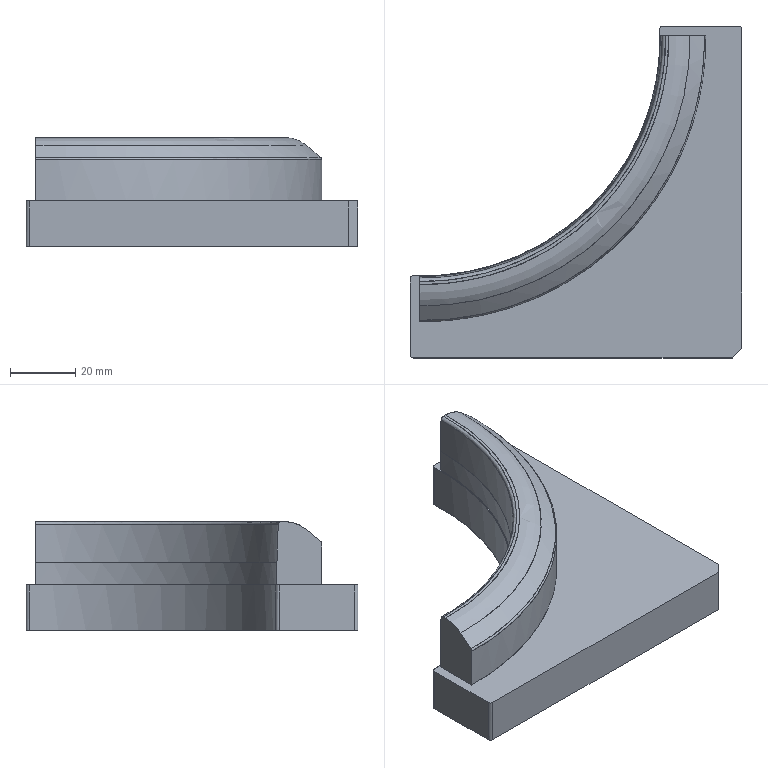NC program | PowerMill | posted with a generic post | part box 102 x 102 x 33.478 mm
Lines 1 to 899 of 321973:
%
O0001
N104 ( POWERMILL CB  : 2026004.0)
N105 ( POST VER      : 2026.0.0.5161)
N106 ( OPTION FILE   : FANUC)
N107 ( OUTPUT WORKPLANE : WORLD)
N108 (  )
N109 ( TOOL LIST )
N110 (---------------------------------------)
N111 ( NO. | ID        | DIA.| TIP RAD|LENGTH)
N112 (---------------------------------------)
N113 (    1|D10C_1_1_1 |10.0 |  0.0   |88.92 )
N114 (    3|D10_1_1_1  |10.0 |  0.0   |88.64 )
N115 (    7|R2_1_1_1   | 4.0 |  2.0   |69.84 )
N116 (   13|TEXT_D4_1_1| 4.0 |  0.3   |74.72 )
N117 (---------------------------------------)
N118 (  )
N119 ( NUMBER OF TOOLPATHS: 11.0 )
N120 ( ESTIMATED PROGRAM DURATION: 1 HOURS 4 MIN 54 SEC)
N121 (  )
N122 G00 G21 G80 G40 G17
N123 G90
N124 G54
N125 G53 Z0.0
N126 (---------------)
N127 ( START TOOLPATH : 精公开粗01-扫面平行-D10C )
N128 (---------------)
N129 ( TOOL NO.    :1 )
N130 ( TOOL TYPE   : ENDMILL)
N131 ( TOOL ID     : D10C_1_1_1)
N132 ( TOOL DIA    : 10.0 LENGTH 88.92)
N133 T1
N134 M6
N135 S8000 M03
N136 G00 G90 X0.0 Y0.0
N137 G43 Z10.2 H1
N138
N139 G05 P10000 R4
N140 X63.78 Y58.78
N141 Z1.128
N142 G01 Z-0.072 F6000.0
N143 X58.78 F10000.0
N144 X-58.78
N145 Y52.902
N146 X58.78
N147 Y47.024
N148 X-58.78
N149 Y41.146
N150 X58.78
N151 Y35.268
N152 X-58.78
N153 Y29.39
N154 X58.78
N155 Y23.512
N156 X-58.78
N157 Y17.634
N158 X58.78
N159 Y11.756
N160 X-58.78
N161 Y5.878
N162 X58.78
N163 Y0.0
N164 X-58.78
N165 Y-5.878
N166 X58.78
N167 Y-11.756
N168 X-58.78
N169 Y-17.634
N170 X58.78
N171 Y-23.512
N172 X-58.78
N173 Y-29.39
N174 X58.78
N175 Y-35.268
N176 X-58.78
N177 Y-41.146
N178 X58.78
N179 Y-47.024
N180 X-58.78
N181 Y-52.902
N182 X58.78
N183 Y-58.78
N184 X-58.78
N185 X-63.78
N186 G00 Z10.2
N187 G05 P0
N188 (---------------)
N189 ( END TOOLPATH : 精公开粗01-扫面平行-D10C )
N190 (---------------)
N191 ( START TOOLPATH : 精公开粗01-外形偏置-D10C )
N192 (---------------)
N193 G00 X0.0 Y0.0 Z9.878
N194 G05 P10000 R4
N195 X24.2557 Y64.055
N196 Z0.6827
N197 G01 Z-0.5173 F6000.0
N198 Y63.5275 F10000.0
N199 G03 X29.0032 Y58.78 I4.7475 J0.0
N200 G01 X58.78
N201 Y-58.78
N202 X-58.78
N203 Y58.78
N204 X29.0032
N205 X29.0035 Y53.28
N206 X30.9371 Y53.2801
N207 X31.7105 Y53.2395
N208 X32.4839 Y53.0979
N209 X33.2573 Y52.8385
N210 X33.7698 Y52.593
N211 X34.0308 Y52.4374
N212 X34.8381 Y51.8196
N213 X35.5147 Y51.0461
N214 X35.9743 Y50.2727
N215 X36.2769 Y49.4993
N216 X36.4465 Y48.7259
N217 X36.4984 Y47.9524
N218 X36.473 Y45.6322
N219 X36.4018 Y43.3119
N220 X36.2632 Y40.9916
N221 X36.0636 Y38.6713
N222 X35.7969 Y36.351
N223 X35.345 Y33.2573
N224 X34.9245 Y30.9371
N225 X34.4344 Y28.6168
N226 X33.8747 Y26.2965
N227 X33.2442 Y23.9762
N228 X32.4839 Y21.4686
N229 X31.7105 Y19.1775
N230 X30.9371 Y17.087
N231 X29.9777 Y14.6951
N232 X28.963 Y12.3748
N233 X27.8434 Y10.0186
N234 X26.672 Y7.7343
N235 X25.5231 Y5.649
N236 X24.4731 Y3.8671
N237 X23.0232 Y1.5469
N238 X21.6559 Y-0.493
N239 X20.1091 Y-2.6583
N240 X18.5622 Y-4.6834
N241 X17.0154 Y-6.588
N242 X15.3542 Y-8.5077
N243 X13.9217 Y-10.0752
N244 X12.4521 Y-11.6014
N245 X12.0183 Y-12.0293
N246 X15.9279 Y-15.9356
N247 X19.4366 Y-19.4412
N248 X23.0192 Y-23.0208
N249 X26.9274 Y-26.9257
N250 X30.1108 Y-30.1063
N251 X26.9274 Y-26.9257
N252 G02 X19.7102 Y-33.5004 I-73.5184 J73.4557
N253 G01 X18.2283 Y-34.728
N254 G03 X19.1615 Y-37.1995 I0.891 J-1.0755
N255 G01 X34.7903 Y-36.7263
N256 G03 X36.7288 Y-34.788 I-0.0606 J1.9991
N257 G01 X37.2052 Y-19.1304
N258 G03 X34.7358 Y-18.2004 I-1.3938 J0.0424
N259 G01 X33.5664 Y-19.6175
N260 G02 X26.9274 Y-26.9257 I-80.158 J66.1482
N261 G01 X23.0192 Y-23.0208
N262 G02 X0.3003 Y-40.0065 I-70.0268 J69.9762
N263 G01 X-1.0304 Y-40.7304
N264 G03 X-0.4806 Y-42.8617 I0.5422 J-0.9967
N265 G01 X40.6034 Y-42.5887
N266 G03 X42.59 Y-40.6024 I-0.0133 J2.0
N267 G01 X42.8712 Y0.5029
N268 G03 X40.7411 Y1.0534 I-1.1342 J0.0077
N269 G01 X39.9453 Y-0.4069
N270 G02 X30.7764 Y-14.2827 I-86.0597 J46.8998
N271 G01 X30.6579 Y-14.4326
N272 G02 X23.0192 Y-23.0208 I-77.6654 J61.3879
N273 G01 X19.4366 Y-19.4412
N274 G02 X-23.4816 Y-43.9834 I-66.4441 J66.3965
N275 G01 X-33.3637 Y-46.5399
N276 G02 X-47.466 Y-47.3641 I-9.1402 J35.3311
N277 G01 X-47.7435 Y-47.326
N278 G03 X-47.942 Y-47.8525 I-0.0392 J-0.2859
N279 G01 X-47.9141 Y-47.871
N280 X-47.8328 Y-47.9091
N281 X-47.744 Y-47.9222
N282 X47.5832 Y-47.941
N283 G03 X47.941 Y-47.5833 I0.0001 J0.3577
N284 G01 Y47.6967
N285 G03 X47.5804 Y48.0723 I-0.3758 J0.0
N286 G01 X47.2764 Y48.0846
N287 G03 X46.9267 Y47.7474 I-0.0136 J-0.3359
N288 G01 X46.9288 Y47.1755
N289 G02 X25.493 Y-12.7692 I-93.565 J-0.3468
N290 G01 X25.4045 Y-12.8763
N291 G02 X19.4366 Y-19.4412 I-72.4118 J59.8314
N292 G01 X15.9279 Y-15.9356
N293 X16.0792 Y-15.7834
N294 X16.2302 Y-15.6309
N295 X16.4169 Y-15.4418
N296 G03 X41.9757 Y47.9407 I-63.0595 J62.2731
N297 G01 X41.9626 Y48.9917
N298 X41.807 Y51.0181
N299 G02 X43.8815 Y53.1739 I1.9938 J0.1574
N300 G01 X50.9699 Y52.8876
N301 G02 X52.8892 Y50.8892 I-0.0807 J-1.9984
N302 G01 Y-50.8892
N303 G02 X50.8892 Y-52.8892 I-2.0 J0.0
N304 G01 X-50.8892
N305 G02 X-52.8875 Y-50.9702 I0.0 J2.0
N306 G01 X-53.1748 Y-43.8839
N307 G02 X-50.8653 Y-41.8272 I1.9984 J0.081
N308 G01 X-47.4068 Y-42.3719
N309 G03 X-34.57 Y-41.7413 I4.9042 J31.1382
N310 G01 X-24.523 Y-39.1289
N311 G03 X15.9279 Y-15.9356 I-22.3008 J85.7655
N312 G01 X12.0183 Y-12.0293
N313 X10.828 Y-13.203
N314 X8.5077 Y-15.3531
N315 X6.9608 Y-16.6948
N316 X4.6406 Y-18.5922
N317 X2.659 Y-20.1091
N318 X0.7734 Y-21.4609
N319 X-1.5469 Y-23.0232
N320 X-3.0937 Y-24.0012
N321 X-5.414 Y-25.3845
N322 X-7.7343 Y-26.672
N323 X-9.2811 Y-27.4702
N324 X-11.6341 Y-28.6168
N325 X-13.9217 Y-29.6458
N326 X-16.242 Y-30.6064
N327 X-18.5622 Y-31.4853
N328 X-21.4686 Y-32.4839
N329 X-23.2028 Y-33.0153
N330 X-25.5231 Y-33.6686
N331 X-28.6168 Y-34.4345
N332 X-30.9371 Y-34.9244
N333 X-33.2573 Y-35.345
N334 X-35.5776 Y-35.6973
N335 X-37.8979 Y-35.9832
N336 X-40.2182 Y-36.2036
N337 X-42.406 Y-36.351
N338 X-43.3119 Y-36.4018
N339 X-45.6322 Y-36.4736
N340 X-47.9524 Y-36.4945
N341 X-48.7259 Y-36.444
N342 X-49.4993 Y-36.2724
N343 X-50.2727 Y-35.9743
N344 X-50.9555 Y-35.5776
N345 X-51.8196 Y-34.8356
N346 X-52.4377 Y-34.0308
N347 X-52.593 Y-33.7692
N348 X-52.8386 Y-33.2573
N349 X-53.0982 Y-32.4839
N350 X-53.2386 Y-31.7105
N351 X-53.28 Y-30.9371
N352 X-53.2799 Y-27.0699
N353 X-53.2563 Y-26.2965
N354 X-53.1275 Y-25.5231
N355 X-52.874 Y-24.7496
N356 X-52.4771 Y-23.9762
N357 X-51.8901 Y-23.2028
N358 X-51.0461 Y-22.4565
N359 X-50.2727 Y-22.0014
N360 X-49.4993 Y-21.7038
N361 X-48.7259 Y-21.5366
N362 X-47.9524 Y-21.4847
N363 X-45.6322 Y-21.4716
N364 X-42.5385 Y-21.3468
N365 X-40.2182 Y-21.1481
N366 X-37.1245 Y-20.7744
N367 X-34.0308 Y-20.249
N368 X-31.7105 Y-19.7625
N369 X-29.3902 Y-19.1832
N370 X-26.2965 Y-18.2876
N371 X-23.9762 Y-17.5023
N372 X-21.6559 Y-16.6223
N373 X-18.9243 Y-15.4685
N374 X-16.242 Y-14.1974
N375 X-13.9217 Y-12.9724
N376 X-11.5494 Y-11.6014
N377 X-9.1079 Y-10.0545
N378 X-6.8752 Y-8.5077
N379 X-4.6406 Y-6.8207
N380 X-2.921 Y-5.414
N381 X-0.7734 Y-3.5349
N382 X1.3109 Y-1.5469
N383 X3.0937 Y0.299
N384 X4.9042 Y2.3203
N385 X6.8201 Y4.6406
N386 X8.5077 Y6.8752
N387 X10.0545 Y9.1075
N388 X11.5458 Y11.4656
N389 X5.9314 Y14.7685
N390 X0.3703 Y18.04
N391 X-5.2122 Y21.3241
N392 X-10.7952 Y24.6085
N393 X-15.5903 Y27.4294
N394 G03 X-17.1961 Y30.0687 I-1.511 J0.8889
N395 G01 X-27.624 Y29.5035
N396 G03 X-29.5128 Y27.6158 I0.1082 J-1.997
N397 G01 X-30.086 Y17.1419
N398 G03 X-27.102 Y15.8113 I1.746 J-0.0956
N399 G01 X-15.8602 Y27.0802
N400 X-15.7142 Y27.2463
N401 X-15.5903 Y27.4294
N402 X-10.7952 Y24.6085
N403 X-10.5216 Y25.0509
N404 X-10.2534 Y25.4964
N405 X-5.8989 Y32.8265
N406 G03 X-7.6605 Y35.8475 I-1.7195 J1.0215
N407 G01 X-33.3539 Y35.3059
N408 G03 X-35.3112 Y33.3498 I0.0422 J-1.9996
N409 G01 X-35.8718 Y7.5843
N410 G03 X-32.8467 Y5.8238 I1.9996 J-0.0435
N411 G01 X-25.5062 Y10.2077
N412 G03 X-10.7952 Y24.6085 I-22.539 J37.7392
N413 G01 X-5.2122 Y21.3241
N414 G03 X-0.5838 Y30.8924 I-42.8331 J26.6228
N415 G01 X2.2833 Y38.8715
N416 G03 X0.3812 Y41.5477 I-1.8821 J0.6763
N417 G01 X-39.1756 Y41.1535
N418 G03 X-41.1556 Y39.1746 I0.0199 J-2.0
N419 G01 X-41.573 Y-0.4889
N420 G03 X-38.8891 Y-2.3893 I1.9999 J-0.021
N421 G01 X-30.7986 Y0.5549
N422 G03 X-5.2122 Y21.3241 I-17.2467 J47.392
N423 G01 X0.3703 Y18.04
N424 G03 X7.8449 Y37.2332 I-48.4155 J29.9069
N425 G01 X9.3261 Y44.9602
N426 G03 X7.3497 Y47.3367 I-1.9642 J0.3765
N427 G01 X-45.03 Y47.0175
N428 G03 X-47.0178 Y45.0304 I0.0122 J-2.0
N429 G01 X-47.3547 Y-7.5365
N430 G03 X-44.9535 Y-9.5087 I1.9999 J-0.0129
N431 G01 X-36.6288 Y-7.804
N432 G03 X0.3703 Y18.04 I-11.4165 J55.7509
N433 G01 X5.9314 Y14.7685
N434 G02 X-38.9097 Y-14.5381 I-53.1915 J32.4284
N435 G01 X-50.9053 Y-16.1606
N436 G02 X-53.1733 Y-14.17 I-0.268 J1.9819
N437 G01 X-52.8892 Y50.8979
N438 G02 X-50.8978 Y52.8892 I2.0 J-0.0087
N439 G01 X14.1787 Y53.1702
N440 G02 X16.1542 Y50.8078 I0.0086 J-2.0
N441 G01 X15.4431 Y46.9481
N442 G03 X14.9177 Y43.091 I40.923 J-7.5395
N443 G01 X14.7927 Y41.684
N444 G02 X5.9314 Y14.7685 I-62.0528 J5.5129
N445 G01 X11.5458 Y11.4656
N446 X11.6316 Y11.6014
N447 X12.9739 Y13.9217
N448 X14.1968 Y16.242
N449 X15.3079 Y18.5622
N450 X16.3102 Y20.8825
N451 X17.5029 Y23.9762
N452 X18.2868 Y26.2965
N453 X18.9724 Y28.6168
N454 X19.7625 Y31.7105
N455 X20.2476 Y34.0308
N456 X20.7744 Y37.1245
N457 X21.0689 Y39.4448
N458 X21.3462 Y42.5385
N459 X21.3467 Y42.5493
N460 X21.4527 Y44.8587
N461 X21.4845 Y47.9524
N462 X21.5366 Y48.7259
N463 X21.6559 Y49.3234
N464 X22.0031 Y50.2727
N465 X22.4294 Y51.0072
N466 X23.1286 Y51.8196
N467 X23.9762 Y52.4767
N468 X24.7496 Y52.8738
N469 X25.5231 Y53.1272
N470 X26.2965 Y53.2563
N471 X27.0699 Y53.2799
N472 X29.0035 Y53.28
N473 X29.0032 Y58.78
N474 G00 Z3.2875
N475 G01 X24.2557 Y64.055
N476 G00 Z0.2875
N477 G01 Z-0.9125 F6000.0
N478 Y63.5275 F10000.0
N479 G03 X29.0032 Y58.78 I4.7475 J0.0
N480 G01 X58.78
N481 Y-58.78
N482 X-58.78
N483 Y58.78
N484 X29.0032
N485 X29.0035 Y53.28
N486 X30.9371 Y53.2801
N487 X31.0614 Y53.2735
N488 X32.4839
N489 X33.2573 Y53.1848
N490 X34.0308 Y52.9836
N491 X34.8042 Y52.6529
N492 X35.5776 Y52.1596
N493 X35.9782 Y51.8196
N494 X36.351 Y51.4315
N495 X36.6513 Y51.0461
N496 X37.1137 Y50.2727
N497 X37.4138 Y49.4993
N498 X37.5827 Y48.7259
N499 X37.6334 Y47.9524
N500 X37.6252 Y45.6322
N501 X37.5537 Y43.3119
N502 X37.4185 Y40.9916
N503 X37.2196 Y38.6713
N504 X36.8615 Y35.5776
N505 X36.512 Y33.2573
N506 X36.095 Y30.9371
N507 X35.5776 Y28.457
N508 X35.0595 Y26.2965
N509 X34.4381 Y23.9762
N510 X33.5043 Y20.8825
N511 X32.7148 Y18.5622
N512 X31.8485 Y16.242
N513 X30.9035 Y13.9217
N514 X29.8771 Y11.6014
N515 X28.7647 Y9.2811
N516 X27.8434 Y7.4888
N517 X26.7092 Y5.414
N518 X25.5231 Y3.3862
N519 X23.8965 Y0.7734
N520 X22.4294 Y-1.4018
N521 X21.2148 Y-3.0937
N522 X19.4528 Y-5.414
N523 X18.1974 Y-6.9608
N524 X16.2093 Y-9.2811
N525 X14.6951 Y-10.9372
N526 X13.1483 Y-12.5371
N527 X12.8412 Y-12.8367
N528 X16.8015 Y-16.7982
N529 X20.0565 Y-20.0541
N530 X23.6371 Y-23.6357
N531 X27.5432 Y-27.5429
N532 X30.7247 Y-30.7253
N533 X27.5432 Y-27.5429
N534 G02 X20.8298 Y-33.6928 I-73.7852 J73.8062
N535 G01 X19.35 Y-34.9342
N536 G03 X20.2987 Y-37.4051 I0.8994 J-1.0722
N537 G01 X34.9596 Y-36.8882
N538 G03 X36.8878 Y-34.9599 I-0.0705 J1.9988
N539 G01 X37.4042 Y-20.3059
N540 G03 X34.933 Y-19.3565 I-1.399 J0.0493
N541 G01 X33.691 Y-20.8361
N542 G02 X27.5432 Y-27.5429 I-79.9322 J67.0987
N543 G01 X23.6371 Y-23.6357
N544 G02 X1.7879 Y-40.1445 I-70.2745 J70.2945
N545 G01 X0.2651 Y-40.994
N546 G03 X0.831 Y-43.1273 I0.5548 J-0.9946
N547 G01 X40.7564 Y-42.737
N548 G03 X42.7368 Y-40.7566 I-0.0195 J1.9999
N549 G01 X43.1257 Y-0.8541
N550 G03 X40.992 Y-0.2875 I-1.1391 J0.0111
N551 G01 X40.1416 Y-1.8101
N552 G02 X23.6371 Y-23.6357 I-86.7789 J48.4688
N553 G01 X20.0565 Y-20.0541
N554 G02 X-26.1056 Y-45.4262 I-66.7541 J66.7731
N555 G01 X-31.0296 Y-46.5266
N556 G03 X-30.8337 Y-48.2807 I0.1936 J-0.8664
N557 G01 X46.0831 Y-48.0778
N558 G03 X48.0778 Y-46.083 I-0.0053 J2.0
N559 G01 X48.2809 Y31.8987
N560 G03 X46.5848 Y32.0466 I-0.8543 J0.0022
N561 G01 X46.3368 Y30.6142
N562 G02 X20.0565 Y-20.0541 I-93.0344 J16.1048
N563 G01 X16.8015 Y-16.7982
N564 G03 X43.1133 Y47.9321 I-63.5143 J63.5304
N565 G01 X43.0993 Y48.9851
N566 X42.9445 Y51.0186
N567 G02 X45.0342 Y53.1722 I1.9939 J0.1559
N568 G01 X50.985 Y52.8869
N569 G02 X52.8892 Y50.8892 I-0.0958 J-1.9977
N570 G01 Y38.9186
N571 X48.3892
N572 X52.8892
N573 Y-50.8892
N574 G02 X50.8892 Y-52.8892 I-2.0 J0.0
N575 G01 X-50.8892
N576 G02 X-52.8887 Y-50.9331 I0.0 J2.0
N577 G01 X-53.0259 Y-44.6924
N578 G02 X-51.1401 Y-43.0085 I1.6621 J0.0366
N579 G01 X-46.9683 Y-43.5751
N580 G03 X-37.1698 Y-43.1674 I3.757 J27.66
N581 G01 X-27.2696 Y-40.9727
N582 G03 X16.8015 Y-16.7982 I-19.4432 J87.7049
N583 G01 X12.8412 Y-12.8367
N584 X10.9367 Y-14.6951
N585 X9.2466 Y-16.242
N586 X7.455 Y-17.7888
N587 X5.414 Y-19.453
N588 X3.5456 Y-20.8825
N589 X1.4022 Y-22.4294
N590 X-0.7734 Y-23.8966
N591 X-3.0937 Y-25.3533
N592 X-4.6889 Y-26.2965
N593 X-6.9608 Y-27.563
N594 X-9.2811 Y-28.7643
N595 X-11.6014 Y-29.8771
N596 X-13.9217 Y-30.9036
N597 X-16.242 Y-31.8485
N598 X-18.5622 Y-32.715
N599 X-20.8825 Y-33.5042
N600 X-23.2028 Y-34.2195
N601 X-25.5231 Y-34.8624
N602 X-27.8434 Y-35.4351
N603 X-30.1636 Y-35.9388
N604 X-33.2573 Y-36.5122
N605 X-35.5776 Y-36.8615
N606 X-37.7476 Y-37.1245
N607 X-40.2182 Y-37.3595
N608 X-42.5385 Y-37.5125
N609 X-45.6322 Y-37.6251
N610 X-47.9524 Y-37.6295
N611 X-48.7259 Y-37.5803
N612 X-49.4993 Y-37.4136
N613 X-50.2727 Y-37.1126
N614 X-51.0461 Y-36.6521
N615 X-51.4272 Y-36.351
N616 X-51.8196 Y-35.9782
N617 X-52.1582 Y-35.5776
N618 X-52.593 Y-34.9163
N619 X-52.9829 Y-34.0308
N620 X-53.185 Y-33.2573
N621 X-53.2728 Y-32.4839
N622 X-53.273 Y-31.0683
N623 X-53.28 Y-30.9371
N624 X-53.2799 Y-27.0699
N625 X-53.2735 Y-26.8601
N626 Y-26.2965
N627 X-53.1784 Y-25.5231
N628 X-52.9617 Y-24.7496
N629 X-52.6097 Y-23.9762
N630 X-52.0808 Y-23.2028
N631 X-51.8196 Y-22.905
N632 X-51.3022 Y-22.4294
N633 X-51.0461 Y-22.2395
N634 X-50.2727 Y-21.7859
N635 X-49.9862 Y-21.6559
N636 X-49.4993 Y-21.4885
N637 X-48.7259 Y-21.3208
N638 X-47.9524 Y-21.2708
N639 X-45.6322 Y-21.2594
N640 X-42.5385 Y-21.1332
N641 X-39.659 Y-20.8825
N642 X-37.1245 Y-20.5615
N643 X-34.4136 Y-20.1091
N644 X-31.7105 Y-19.5465
N645 X-29.3902 Y-18.9641
N646 X-26.2965 Y-18.0631
N647 X-23.9762 Y-17.279
N648 X-21.2598 Y-16.242
N649 X-18.5622 Y-15.0719
N650 X-16.242 Y-13.9586
N651 X-13.9217 Y-12.7329
N652 X-11.6014 Y-11.3872
N653 X-9.2811 Y-9.9158
N654 X-6.9608 Y-8.3074
N655 X-5.1735 Y-6.9608
N656 X-3.0937 Y-5.282
N657 X-0.7734 Y-3.2494
N658 X1.0052 Y-1.5469
N659 X3.0937 Y0.6047
N660 X4.6217 Y2.3203
N661 X6.5474 Y4.6406
N662 X8.3071 Y6.9608
N663 X9.9165 Y9.2811
N664 X11.3034 Y11.4698
N665 X5.6888 Y14.7731
N666 X0.1222 Y18.0483
N667 X-5.4528 Y21.3284
N668 X-11.0361 Y24.6133
N669 X-15.8302 Y27.4339
N670 G03 X-17.4345 Y30.0681 I-1.5079 J0.8873
N671 G01 X-27.6274 Y29.5059
N672 G03 X-29.5141 Y27.6201 I0.1102 J-1.997
N673 G01 X-30.084 Y17.3856
N674 G03 X-27.1056 Y16.0556 I1.7428 J-0.0971
N675 G01 X-16.0996 Y27.0853
N676 X-15.9539 Y27.2511
N677 X-15.8302 Y27.4339
N678 X-11.0361 Y24.6133
N679 X-10.7492 Y25.0742
N680 X-10.4681 Y25.5386
N681 X-6.1184 Y32.8243
N682 G03 X-7.8782 Y35.849 I-1.7173 J1.0252
N683 G01 X-33.355 Y35.3075
N684 G03 X-35.312 Y33.3518 I0.0425 J-1.9995
N685 G01 X-35.8718 Y7.8091
N686 G03 X-32.8434 Y6.0502 I1.9996 J-0.0438
N687 G01 X-25.5471 Y10.4273
N688 G03 X-11.0361 Y24.6133 I-22.538 J37.569
N689 G01 X-5.4528 Y21.3284
N690 G03 X-0.6879 Y31.1977 I-42.6323 J26.668
N691 G01 X2.037 Y38.8859
N692 G03 X0.1315 Y41.5539 I-1.8851 J0.6681
N693 G01 X-39.1761 Y41.1542
N694 G03 X-41.1557 Y39.1757 I0.0203 J-1.9999
N695 G01 X-41.5771 Y-0.2351
N696 G03 X-38.9007 Y-2.1386 I1.9999 J-0.0214
N697 G01 X-31.0738 Y0.675
N698 G03 X-5.4528 Y21.3284 I-17.0113 J47.3214
N699 G01 X0.1222 Y18.0483
N700 G03 X7.512 Y36.8558 I-47.9527 J29.6968
N701 G01 X9.1053 Y44.9537
N702 G03 X7.1306 Y47.3398 I-1.9623 J0.3861
N703 G01 X-45.0302 Y47.0179
N704 G03 X-47.0178 Y45.0308 I0.0124 J-1.9999
N705 G01 X-47.3548 Y-7.3197
N706 G03 X-44.9422 Y-9.2895 I2.0 J-0.0129
N707 G01 X-36.194 Y-7.445
N708 G03 X0.1222 Y18.0483 I-11.6365 J55.1901
N709 G01 X5.6888 Y14.7731
N710 G02 X-38.9084 Y-14.3197 I-52.9306 J32.4104
N711 G01 X-50.9048 Y-15.9451
N712 G02 X-53.1733 Y-13.9545 I-0.2685 J1.9819
N713 G01 X-52.8892 Y50.8979
N714 G02 X-50.898 Y52.8892 I2.0 J-0.0087
N715 G01 X13.949 Y53.1746
N716 G02 X15.9254 Y50.8161 I0.0088 J-2.0
N717 G01 X15.2189 Y46.9382
N718 G03 X14.7081 Y43.149 I40.6867 J-7.413
N719 G01 X14.5847 Y41.7452
N720 G02 X5.6888 Y14.7731 I-61.8265 J5.4383
N721 G01 X11.3034 Y11.4698
N722 X11.3868 Y11.6014
N723 X12.7329 Y13.9217
N724 X13.958 Y16.242
N725 X15.0714 Y18.5622
N726 X16.242 Y21.2602
N727 X17.2794 Y23.9762
N728 X18.063 Y26.2965
N729 X18.7513 Y28.6168
N730 X19.5461 Y31.7105
N731 X20.1091 Y34.4134
N732 X20.562 Y37.1245
N733 X20.8825 Y39.6585
N734 X21.1332 Y42.5385
N735 X21.1336 Y42.5484
N736 X21.2419 Y44.8587
N737 X21.2716 Y47.9524
N738 X21.3226 Y48.7259
N739 X21.4863 Y49.4993
N740 X21.6559 Y49.9853
N741 X21.7829 Y50.2727
N742 X22.2365 Y51.0461
N743 X22.4294 Y51.301
N744 X22.9076 Y51.8196
N745 X23.2028 Y52.0825
N746 X23.949 Y52.593
N747 X24.7496 Y52.962
N748 X25.5231 Y53.1784
N749 X26.2965 Y53.2737
N750 X26.8654 Y53.2736
N751 X27.0699 Y53.2799
N752 X29.0035 Y53.28
N753 X29.0032 Y58.78
N754 G00 Z2.8922
N755 G01 X24.2557 Y64.055
N756 G00 Z-0.1078
N757 G01 Z-1.3078 F6000.0
N758 Y63.5275 F10000.0
N759 G03 X29.0032 Y58.78 I4.7475 J0.0
N760 G01 X58.78
N761 Y-58.78
N762 X32.3091
N763 X32.0834 Y-52.8892
N764 X31.9005 Y-48.1173
N765 X31.6979 Y-42.8305
N766 X31.4754 Y-37.0245
N767 X31.3031 Y-32.5278
N768 X31.4754 Y-37.0245
N769 X34.9685 Y-36.8906
N770 G03 X36.8905 Y-34.9687 I-0.0765 J1.9985
N771 G01 X37.4015 Y-21.629
N772 G03 X34.9233 Y-20.6592 I-1.4078 J0.0539
N773 G01 X33.6652 Y-22.1295
N774 G02 X22.1291 Y-33.6656 I-79.9039 J68.3678
N775 G01 X20.6588 Y-34.9236
N776 G03 X21.6287 Y-37.4018 I0.9159 J-1.0705
N777 G01 X31.4754 Y-37.0245
N778 X31.6979 Y-42.8305
N779 X40.7581 Y-42.7375
N780 G03 X42.7375 Y-40.7581 I-0.0205 J1.9999
N781 G01 X43.1285 Y-2.5973
N782 G03 X40.9829 Y-2.0094 I-1.1501 J0.0118
N783 G01 X40.104 Y-3.5283
N784 G02 X3.5275 Y-40.1047 I-86.8065 J50.2305
N785 G01 X2.0086 Y-40.9836
N786 G03 X2.5964 Y-43.1291 I0.576 J-0.9955
N787 G01 X31.6979 Y-42.8305
N788 X31.9005 Y-48.1173
N789 X46.0834 Y-48.0778
N790 G03 X48.0778 Y-46.0833 I-0.0056 J2.0
N791 G01 X48.2808 Y27.0645
N792 G03 X46.547 Y27.26 I-0.8777 J0.0025
N793 G01 X46.2183 Y25.8023
N794 G02 X-23.8565 Y-45.7583 I-92.9876 J20.9667
N795 G01 X-26.8916 Y-46.5099
N796 G03 X-26.6731 Y-48.2807 I0.216 J-0.8722
N797 G01 X31.9005 Y-48.1173
N798 X32.0834 Y-52.8892
N799 X-50.8892
N800 G02 X-52.886 Y-51.0016 I0.0 J2.0
N801 G01 X-53.1737 Y-45.8934
N802 G02 X-50.869 Y-43.8048 I1.9968 J0.1125
N803 G01 X-47.4326 Y-44.3403
N804 G03 X-35.2992 Y-43.8222 I4.7707 J30.616
N805 G01 X-25.2248 Y-41.3578
N806 G03 X43.9477 Y47.9257 I-21.5619 J88.1427
N807 G01 X43.9344 Y48.9833
N808 X43.7786 Y51.0194
N809 G02 X45.8845 Y53.1731 I1.9938 J0.1569
N810 G01 X51.0012 Y52.886
N811 G02 X52.8892 Y50.8892 I-0.112 J-1.9968
N812 G01 Y-50.8892
N813 G02 X50.8892 Y-52.8892 I-2.0 J0.0
N814 G01 X32.0834
N815 X32.3091 Y-58.78
N816 X-58.78
N817 Y58.78
N818 X29.0032
N819 X29.0035 Y53.2799
N820 X30.9371 Y53.28
N821 X31.0035 Y53.2765
N822 X33.2573 Y53.2768
N823 X34.0308 Y53.2006
N824 X34.8042 Y53.01
N825 X35.5776 Y52.6909
N826 X36.351 Y52.2105
N827 X36.8176 Y51.8196
N828 X37.1245 Y51.5061
N829 X37.4927 Y51.0461
N830 X37.8979 Y50.3765
N831 X38.2489 Y49.4993
N832 X38.4178 Y48.7259
N833 X38.4681 Y47.9524
N834 X38.4588 Y45.6322
N835 X38.3877 Y43.3119
N836 X38.2535 Y40.9916
N837 X37.9822 Y37.8979
N838 X37.7025 Y35.5776
N839 X37.3552 Y33.2573
N840 X36.9423 Y30.9371
N841 X36.351 Y28.0876
N842 X35.7265 Y25.5231
N843 X35.0897 Y23.2028
N844 X34.3802 Y20.8825
N845 X33.5977 Y18.5622
N846 X32.7404 Y16.242
N847 X31.7105 Y13.6875
N848 X30.7913 Y11.6014
N849 X29.6936 Y9.2811
N850 X28.5092 Y6.9608
N851 X27.2332 Y4.6406
N852 X26.2965 Y3.0517
N853 X24.883 Y0.7734
N854 X23.2028 Y-1.7476
N855 X21.6822 Y-3.8671
N856 X20.1091 Y-5.9274
N857 X18.5622 Y-7.8327
N858 X17.0154 Y-9.6288
N859 X15.2145 Y-11.6014
N860 X13.7168 Y-13.1483
N861 X11.6014 Y-15.2138
N862 X10.0545 Y-16.6319
N863 X7.7343 Y-18.643
N864 X5.9274 Y-20.1091
N865 X3.8671 Y-21.6821
N866 X1.7493 Y-23.2028
N867 X0.0 Y-24.3824
N868 X-2.3203 Y-25.8602
N869 X-4.6406 Y-27.2335
N870 X-6.9608 Y-28.5092
N871 X-8.5077 Y-29.3044
N872 X-10.828 Y-30.4311
N873 X-13.691 Y-31.7105
N874 X-15.4685 Y-32.4346
N875 X-18.5622 Y-33.5977
N876 X-20.8825 Y-34.3803
N877 X-23.2028 Y-35.0897
N878 X-25.5231 Y-35.7265
N879 X-28.0898 Y-36.351
N880 X-30.1636 Y-36.7909
N881 X-32.4839 Y-37.2222
N882 X-35.5776 Y-37.7028
N883 X-37.1981 Y-37.8979
N884 X-37.8979 Y-37.9824
N885 X-40.2182 Y-38.1966
N886 X-42.5385 Y-38.3476
N887 X-45.6322 Y-38.4588
N888 X-47.9524 Y-38.4695
N889 X-48.7259 Y-38.4196
N890 X-49.4993 Y-38.2503
N891 X-50.2727 Y-37.9514
N892 X-51.0461 Y-37.4937
N893 X-51.5057 Y-37.1245
N894 X-51.8196 Y-36.818
N895 X-52.2104 Y-36.351
N896 X-52.6895 Y-35.5776
N897 X-53.01 Y-34.8042
N898 X-53.2001 Y-34.0308
N899 X-53.2774 Y-33.2573
N900 X-53.2769 Y-30.9937
N901 X-53.2799 Y-30.9371
N902 Y-27.0699
N903 X-53.276 Y-26.9429
N904 X-53.2758 Y-26.2965
N905 X-53.1853 Y-25.5231
N906 X-52.9786 Y-24.7496
N907 X-52.6363 Y-23.9762
N908 X-52.1242 Y-23.2028
N909 X-51.8196 Y-22.8549
N910 X-51.3633 Y-22.4294
N911 X-51.0461 Y-22.1874
N912 X-50.2727 Y-21.7337
N913 X-49.4993 Y-21.4369
N914 X-48.7259 Y-21.2696
N915 X-47.9524 Y-21.2195
N916 X-45.6322 Y-21.2044
N917 X-42.5385 Y-21.0791
N918 X-40.2182 Y-20.8798
N919 X-37.1245 Y-20.5056
N920 X-34.8042 Y-20.1194
N921 X-31.7105 Y-19.49
N922 X-29.3902 Y-18.9074
N923 X-26.2965 Y-18.005
N924 X-23.9762 Y-17.2209
N925 X-21.409 Y-16.242
N926 X-18.5622 Y-15.0104
N927 X-16.242 Y-13.8957
N928 X-13.9217 Y-12.6703
N929 X-11.6014 Y-11.3237
N930 X-9.2811 Y-9.8502
N931 X-6.9608 Y-8.2391
N932 X-5.2649 Y-6.9608
N933 X-3.0937 Y-5.2105
N934 X-0.6841 Y-3.0937
N935 X0.9264 Y-1.5469
N936 X3.0937 Y0.6835
N937 X5.2119 Y3.0937
N938 X6.4757 Y4.6406
N939 X8.2393 Y6.9608
N940 X9.8518 Y9.2811
N941 X11.2459 Y11.4787
N942 X5.6273 Y14.784
N943 X0.0644 Y18.0564
N944 X-5.5185 Y21.3406
N945 X-11.1018 Y24.6251
N946 X-15.8955 Y27.445
N947 G03 X-17.5027 Y30.0812 I-1.5093 J0.8879
N948 G01 X-27.6291 Y29.5138
N949 G03 X-29.5141 Y27.6291 I0.1119 J-1.9969
N950 G01 X-30.0852 Y17.4647
N951 G03 X-27.1045 Y16.1328 I1.7441 J-0.098
N952 G01 X-16.1652 Y27.096
N953 X-16.0193 Y27.262
N954 X-15.8955 Y27.445
N955 X-11.1018 Y24.6251
N956 X-10.8098 Y25.0953
N957 X-10.5239 Y25.5692
N958 X-6.1955 Y32.8457
N959 G03 X-7.9581 Y35.8676 I-1.7189 J1.0224
N960 G01 X-33.3555 Y35.3128
N961 G03 X-35.3114 Y33.3575 I0.0436 J-1.9996
N962 G01 X-35.8749 Y7.8971
N963 G03 X-32.8485 Y6.1366 I1.9995 J-0.0442
N964 G01 X-25.5514 Y10.5028
N965 G03 X-11.1018 Y24.6251 I-22.3002 J37.2702
N966 G01 X-5.5185 Y21.3406
N967 G03 X-0.8561 Y30.9745 I-42.3331 J26.4324
N968 G01 X1.9771 Y38.9007
N969 G03 X0.0726 Y41.5738 I-1.8833 J0.6732
N970 G01 X-39.1766 Y41.1572
N971 G03 X-41.1552 Y39.1788 I0.0212 J-1.9999
N972 G01 X-41.577 Y-0.182
N973 G03 X-38.8919 Y-2.0824 I1.9999 J-0.0214
N974 G01 X-30.7521 Y0.8862
N975 G03 X-5.5185 Y21.3406 I-17.0995 J46.8868
N976 G01 X0.0644 Y18.0564
N977 G03 X7.5558 Y37.3308 I-47.916 J29.7166
N978 G01 X9.0009 Y44.9987
N979 G03 X7.022 Y47.3691 I-1.9654 J0.3704
N980 G01 X-45.0313 Y47.018
N981 G03 X-47.0178 Y45.0309 I0.0135 J-2.0
N982 G01 X-47.3545 Y-7.2679
N983 G03 X-44.9415 Y-9.2377 I1.9999 J-0.0129
N984 G01 X-36.208 Y-7.3944
N985 G03 X0.0644 Y18.0564 I-11.6436 J55.1674
N986 G01 X5.6273 Y14.784
N987 G02 X-38.916 Y-14.269 I-52.8676 J32.3825
N988 G01 X-50.9045 Y-15.8934
N989 G02 X-53.173 Y-13.9027 I-0.2686 J1.9819
N990 G01 X-52.8892 Y50.8979
N991 G02 X-50.898 Y52.8892 I2.0 J-0.0087
N992 G01 X13.9035 Y53.1751
N993 G02 X15.8789 Y50.8112 I0.0088 J-2.0
N994 G01 X15.1667 Y46.9623
N995 G03 X14.6566 Y43.2911 I40.5709 J-7.5083
N996 G01 X14.3651 Y40.171